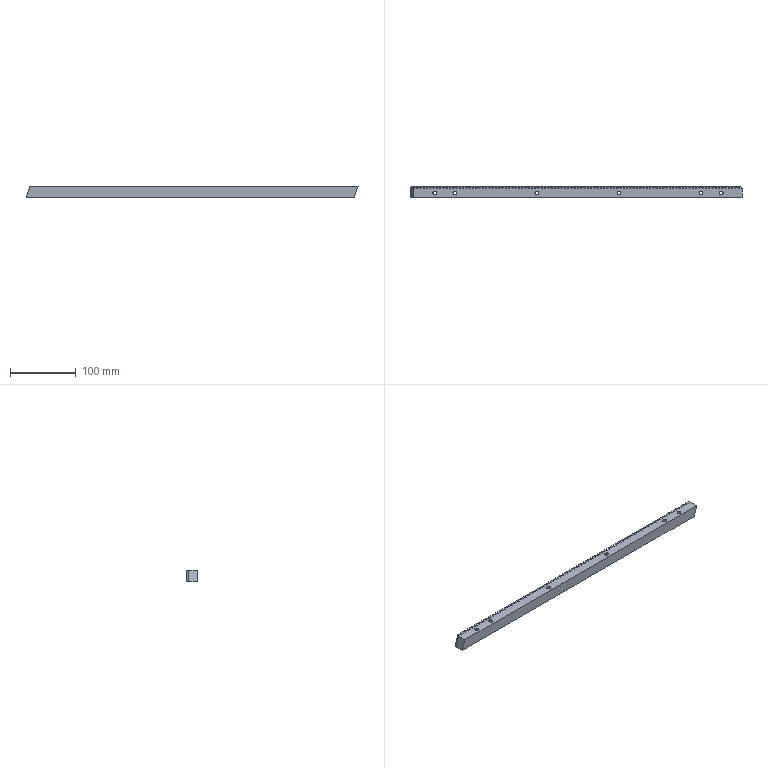Part | SolidWorks | features MirrorStock 1 | 1 solid | 430 faces | box 506 x 17 x 17 mm | volume 126996 mm3 | plane 410 | cylinder 20 | commonest cylinder face diameters 6 x8 9.5 x8 5.7 x4